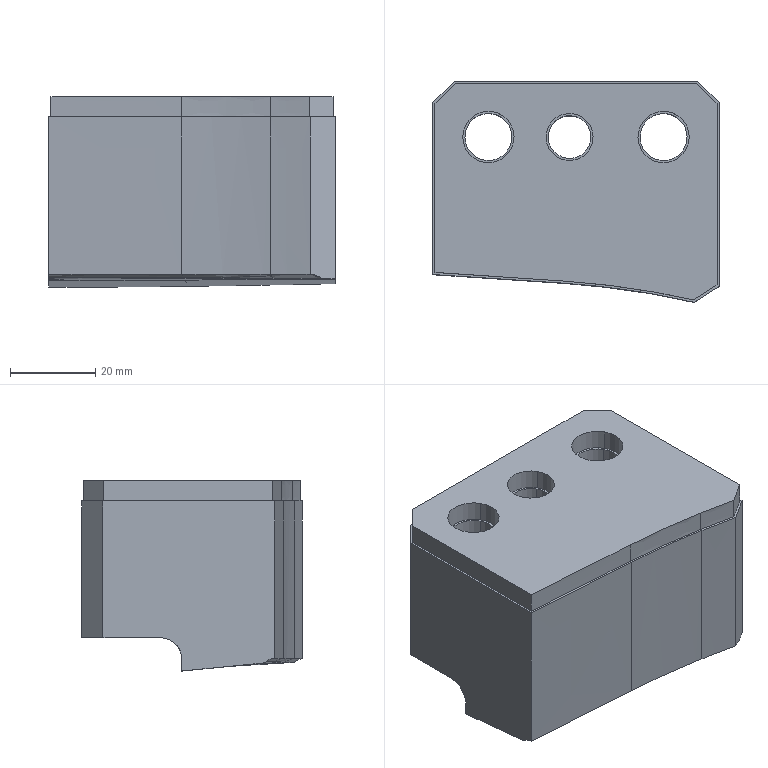Part | CATIA | 2 solids | 66 faces | box 67 x 51.664 x 44.519 mm | volume 110677 mm3 | plane 22 | cylinder 20 | spline 17 | other 7 | commonest cylinder face diameters 11 x6 10 x5 12 x4 18 x4 394.263 x1